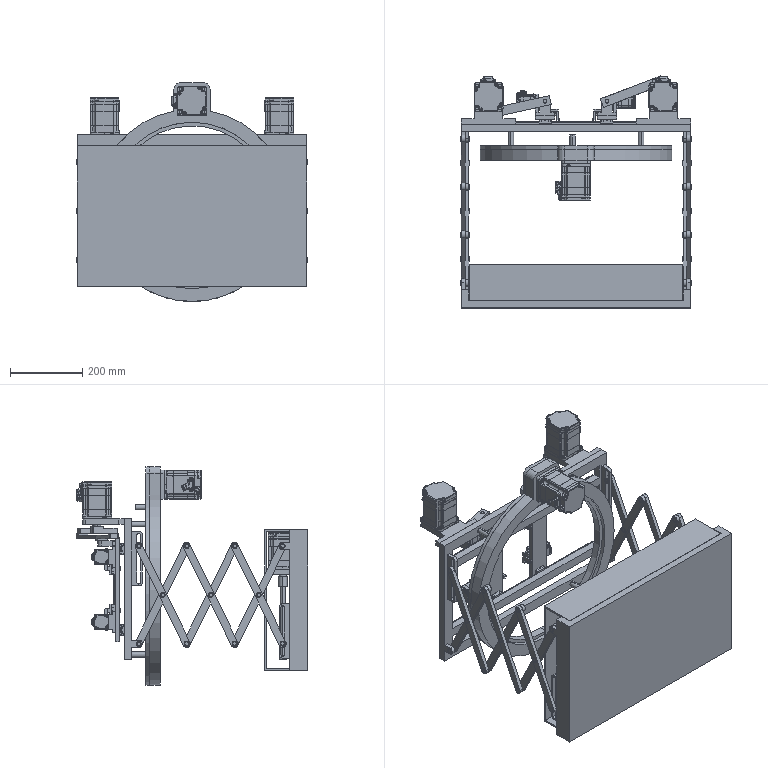Part | SolidWorks | 80 solids | 11673 faces | volume 16381446 mm3 | plane 4399 | cylinder 4250 | spline 1858 | cone 682 | torus 484 | commonest cylinder face diameters 0.6 x351 3 x260 1 x240 6 x236 4 x228 0.5 x224